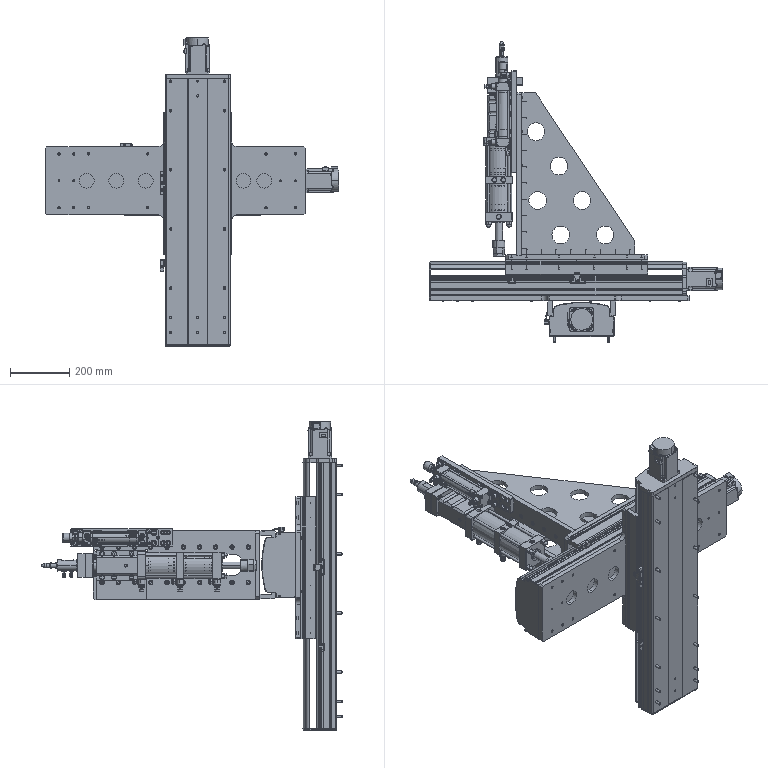Part | SolidWorks | features ReferencePattern 84, LocalLPattern 9, CompositeCurve 3 | 261 solids | 8367 faces | volume 39845939 mm3 | plane 3599 | cylinder 3132 | cone 964 | torus 606 | spline 54 | sphere 12 | commonest cylinder face diameters 15 x296 8 x266 13 x238 6.8 x170 8.6 x168 9 x163